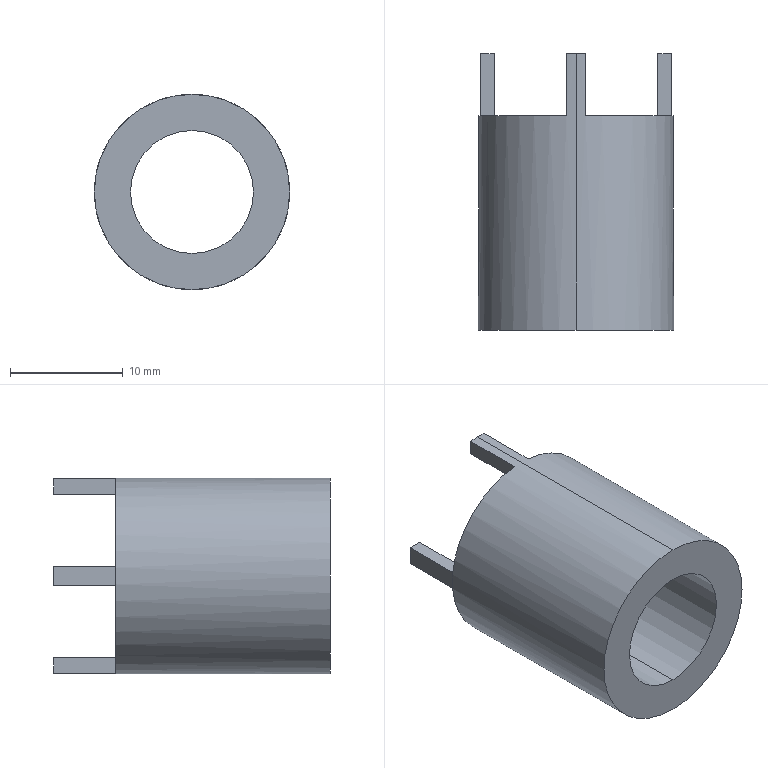Part | STEP file | 1 solid | 27 faces | box 17.3 x 24.5 x 17.3 mm | volume 2659 mm3 | plane 21 | cylinder 6 | commonest cylinder face diameters 10.9 x2 13.1 x2 17.3 x2